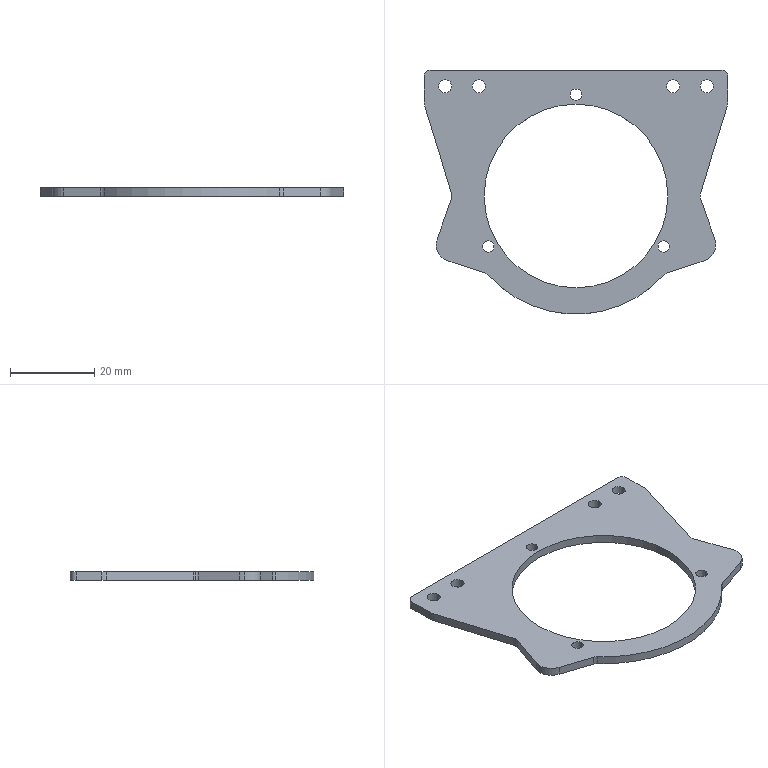Part | SolidWorks | features Fillet 3, Extrusion 1 | 1 solid | 40 faces | box 72 x 57.8 x 2 mm | volume 3745 mm3 | cylinder 29 | plane 11 | commonest cylinder face diameters 3.1 x8 2.7 x6 4 x5 8 x5 3 x2 43.5 x2
STEP:
#1=CARTESIAN_POINT('',(-33.109,-11.571,2.));
#2=VERTEX_POINT('',#1);
#3=CARTESIAN_POINT('',(-30.345,-15.376,2.));
#4=VERTEX_POINT('',#3);
#5=CARTESIAN_POINT('',(-29.109,-11.571,2.));
#6=DIRECTION('',(0.,0.,1.));
#7=DIRECTION('',(1.,0.,0.));
#8=AXIS2_PLACEMENT_3D('',#5,#6,#7);
#9=CIRCLE('',#8,4.);
#10=EDGE_CURVE('',#2,#4,#9,.T.);
#11=ORIENTED_EDGE('',*,*,#10,.F.);
#12=CARTESIAN_POINT('',(-33.109,-11.571,0.));
#13=VERTEX_POINT('',#12);
#14=CARTESIAN_POINT('',(-33.109,-11.571,2.));
#15=DIRECTION('',(0.,0.,-1.));
#16=VECTOR('',#15,1000.);
#17=LINE('',#14,#16);
#18=EDGE_CURVE('',#2,#13,#17,.T.);
#19=ORIENTED_EDGE('',*,*,#18,.T.);
#20=CARTESIAN_POINT('',(-30.345,-15.376,0.));
#21=VERTEX_POINT('',#20);
#22=CARTESIAN_POINT('',(-29.109,-11.571,0.));
#23=DIRECTION('',(0.,0.,-1.));
#24=DIRECTION('',(1.,0.,0.));
#25=AXIS2_PLACEMENT_3D('',#22,#23,#24);
#26=CIRCLE('',#25,4.);
#27=EDGE_CURVE('',#21,#13,#26,.T.);
#28=ORIENTED_EDGE('',*,*,#27,.F.);
#29=CARTESIAN_POINT('',(-30.345,-15.376,2.));
#30=DIRECTION('',(0.,0.,-1.));
#31=VECTOR('',#30,1000.);
#32=LINE('',#29,#31);
#33=EDGE_CURVE('',#4,#21,#32,.T.);
#34=ORIENTED_EDGE('',*,*,#33,.F.);
#35=EDGE_LOOP('',(#11,#19,#28,#34));
#36=FACE_OUTER_BOUND('',#35,.T.);
#37=CARTESIAN_POINT('',(-29.109,-11.571,2.));
#38=DIRECTION('',(0.,0.,-1.));
#39=DIRECTION('',(-1.,0.,0.));
#40=AXIS2_PLACEMENT_3D('',#37,#38,#39);
#41=CYLINDRICAL_SURFACE('',#40,4.);
#42=ADVANCED_FACE('',(#36),#41,.T.);
#43=CARTESIAN_POINT('',(-29.4,0.04046,0.));
#44=VERTEX_POINT('',#43);
#45=CARTESIAN_POINT('',(-29.488,0.6284,0.));
#46=VERTEX_POINT('',#45);
#47=CARTESIAN_POINT('',(-31.4,0.04046,0.));
#48=DIRECTION('',(0.,0.,1.));
#49=DIRECTION('',(1.,0.,0.));
#50=AXIS2_PLACEMENT_3D('',#47,#48,#49);
#51=CIRCLE('',#50,2.);
#52=EDGE_CURVE('',#44,#46,#51,.T.);
#53=ORIENTED_EDGE('',*,*,#52,.F.);
#54=CARTESIAN_POINT('',(-29.4,0.04046,2.));
#55=VERTEX_POINT('',#54);
#56=CARTESIAN_POINT('',(-29.4,0.04046,2.));
#57=DIRECTION('',(0.,0.,1.));
#58=VECTOR('',#57,1000.);
#59=LINE('',#56,#58);
#60=EDGE_CURVE('',#44,#55,#59,.T.);
#61=ORIENTED_EDGE('',*,*,#60,.T.);
#62=CARTESIAN_POINT('',(-29.488,0.6284,2.));
#63=VERTEX_POINT('',#62);
#64=CARTESIAN_POINT('',(-31.4,0.04046,2.));
#65=DIRECTION('',(0.,0.,-1.));
#66=DIRECTION('',(1.,0.,0.));
#67=AXIS2_PLACEMENT_3D('',#64,#65,#66);
#68=CIRCLE('',#67,2.);
#69=EDGE_CURVE('',#63,#55,#68,.T.);
#70=ORIENTED_EDGE('',*,*,#69,.F.);
#71=CARTESIAN_POINT('',(-29.488,0.6284,2.));
#72=DIRECTION('',(0.,0.,1.));
#73=VECTOR('',#72,1000.);
#74=LINE('',#71,#73);
#75=EDGE_CURVE('',#46,#63,#74,.T.);
#76=ORIENTED_EDGE('',*,*,#75,.F.);
#77=EDGE_LOOP('',(#53,#61,#70,#76));
#78=FACE_OUTER_BOUND('',#77,.T.);
#79=CARTESIAN_POINT('',(-31.4,0.04046,2.));
#80=DIRECTION('',(0.,0.,1.));
#81=DIRECTION('',(1.,0.,0.));
#82=AXIS2_PLACEMENT_3D('',#79,#80,#81);
#83=CYLINDRICAL_SURFACE('',#82,2.);
#84=ADVANCED_FACE('',(#78),#83,.F.);
#85=CARTESIAN_POINT('',(-22.135,-12.,2.));
#86=VERTEX_POINT('',#85);
#87=CARTESIAN_POINT('',(-19.435,-12.,2.));
#88=VERTEX_POINT('',#87);
#89=CARTESIAN_POINT('',(-20.785,-12.,2.));
#90=DIRECTION('',(0.,0.,1.));
#91=DIRECTION('',(1.,0.,0.));
#92=AXIS2_PLACEMENT_3D('',#89,#90,#91);
#93=CIRCLE('',#92,1.35);
#94=EDGE_CURVE('',#86,#88,#93,.T.);
#95=ORIENTED_EDGE('',*,*,#94,.T.);
#96=CARTESIAN_POINT('',(-19.435,-12.,0.));
#97=VERTEX_POINT('',#96);
#98=CARTESIAN_POINT('',(-19.435,-12.,2.));
#99=DIRECTION('',(0.,0.,-1.));
#100=VECTOR('',#99,1000.);
#101=LINE('',#98,#100);
#102=EDGE_CURVE('',#88,#97,#101,.T.);
#103=ORIENTED_EDGE('',*,*,#102,.T.);
#104=CARTESIAN_POINT('',(-22.135,-12.,0.));
#105=VERTEX_POINT('',#104);
#106=CARTESIAN_POINT('',(-20.785,-12.,0.));
#107=DIRECTION('',(0.,0.,1.));
#108=DIRECTION('',(1.,0.,0.));
#109=AXIS2_PLACEMENT_3D('',#106,#107,#108);
#110=CIRCLE('',#109,1.35);
#111=EDGE_CURVE('',#105,#97,#110,.T.);
#112=ORIENTED_EDGE('',*,*,#111,.F.);
#113=CARTESIAN_POINT('',(-22.135,-12.,2.));
#114=DIRECTION('',(0.,0.,-1.));
#115=VECTOR('',#114,1000.);
#116=LINE('',#113,#115);
#117=EDGE_CURVE('',#86,#105,#116,.T.);
#118=ORIENTED_EDGE('',*,*,#117,.F.);
#119=EDGE_LOOP('',(#95,#103,#112,#118));
#120=FACE_OUTER_BOUND('',#119,.T.);
#121=CARTESIAN_POINT('',(-20.785,-12.,2.));
#122=DIRECTION('',(0.,0.,-1.));
#123=DIRECTION('',(-1.,0.,0.));
#124=AXIS2_PLACEMENT_3D('',#121,#122,#123);
#125=CYLINDRICAL_SURFACE('',#124,1.35);
#126=ADVANCED_FACE('',(#120),#125,.F.);
#127=CARTESIAN_POINT('',(19.435,-12.,2.));
#128=VERTEX_POINT('',#127);
#129=CARTESIAN_POINT('',(22.135,-12.,2.));
#130=VERTEX_POINT('',#129);
#131=CARTESIAN_POINT('',(20.785,-12.,2.));
#132=DIRECTION('',(0.,0.,1.));
#133=DIRECTION('',(1.,0.,0.));
#134=AXIS2_PLACEMENT_3D('',#131,#132,#133);
#135=CIRCLE('',#134,1.35);
#136=EDGE_CURVE('',#128,#130,#135,.T.);
#137=ORIENTED_EDGE('',*,*,#136,.T.);
#138=CARTESIAN_POINT('',(22.135,-12.,0.));
#139=VERTEX_POINT('',#138);
#140=CARTESIAN_POINT('',(22.135,-12.,2.));
#141=DIRECTION('',(0.,0.,-1.));
#142=VECTOR('',#141,1000.);
#143=LINE('',#140,#142);
#144=EDGE_CURVE('',#130,#139,#143,.T.);
#145=ORIENTED_EDGE('',*,*,#144,.T.);
#146=CARTESIAN_POINT('',(19.435,-12.,0.));
#147=VERTEX_POINT('',#146);
#148=CARTESIAN_POINT('',(20.785,-12.,0.));
#149=DIRECTION('',(0.,0.,1.));
#150=DIRECTION('',(1.,0.,0.));
#151=AXIS2_PLACEMENT_3D('',#148,#149,#150);
#152=CIRCLE('',#151,1.35);
#153=EDGE_CURVE('',#147,#139,#152,.T.);
#154=ORIENTED_EDGE('',*,*,#153,.F.);
#155=CARTESIAN_POINT('',(19.435,-12.,2.));
#156=DIRECTION('',(0.,0.,-1.));
#157=VECTOR('',#156,1000.);
#158=LINE('',#155,#157);
#159=EDGE_CURVE('',#128,#147,#158,.T.);
#160=ORIENTED_EDGE('',*,*,#159,.F.);
#161=EDGE_LOOP('',(#137,#145,#154,#160));
#162=FACE_OUTER_BOUND('',#161,.T.);
#163=CARTESIAN_POINT('',(20.785,-12.,2.));
#164=DIRECTION('',(0.,0.,-1.));
#165=DIRECTION('',(-1.,0.,0.));
#166=AXIS2_PLACEMENT_3D('',#163,#164,#165);
#167=CYLINDRICAL_SURFACE('',#166,1.35);
#168=ADVANCED_FACE('',(#162),#167,.F.);
#169=CARTESIAN_POINT('',(29.45,26.,2.));
#170=VERTEX_POINT('',#169);
#171=CARTESIAN_POINT('',(32.55,26.,2.));
#172=VERTEX_POINT('',#171);
#173=CARTESIAN_POINT('',(31.,26.,2.));
#174=DIRECTION('',(0.,0.,1.));
#175=DIRECTION('',(-1.,0.,0.));
#176=AXIS2_PLACEMENT_3D('',#173,#174,#175);
#177=CIRCLE('',#176,1.55);
#178=EDGE_CURVE('',#170,#172,#177,.T.);
#179=ORIENTED_EDGE('',*,*,#178,.T.);
#180=CARTESIAN_POINT('',(32.55,26.,0.));
#181=VERTEX_POINT('',#180);
#182=CARTESIAN_POINT('',(32.55,26.,2.));
#183=DIRECTION('',(0.,0.,-1.));
#184=VECTOR('',#183,1000.);
#185=LINE('',#182,#184);
#186=EDGE_CURVE('',#172,#181,#185,.T.);
#187=ORIENTED_EDGE('',*,*,#186,.T.);
#188=CARTESIAN_POINT('',(29.45,26.,0.));
#189=VERTEX_POINT('',#188);
#190=CARTESIAN_POINT('',(31.,26.,0.));
#191=DIRECTION('',(0.,0.,1.));
#192=DIRECTION('',(-1.,0.,0.));
#193=AXIS2_PLACEMENT_3D('',#190,#191,#192);
#194=CIRCLE('',#193,1.55);
#195=EDGE_CURVE('',#189,#181,#194,.T.);
#196=ORIENTED_EDGE('',*,*,#195,.F.);
#197=CARTESIAN_POINT('',(29.45,26.,2.));
#198=DIRECTION('',(0.,0.,-1.));
#199=VECTOR('',#198,1000.);
#200=LINE('',#197,#199);
#201=EDGE_CURVE('',#170,#189,#200,.T.);
#202=ORIENTED_EDGE('',*,*,#201,.F.);
#203=EDGE_LOOP('',(#179,#187,#196,#202));
#204=FACE_OUTER_BOUND('',#203,.T.);
#205=CARTESIAN_POINT('',(31.,26.,2.));
#206=DIRECTION('',(0.,0.,-1.));
#207=DIRECTION('',(-1.,0.,0.));
#208=AXIS2_PLACEMENT_3D('',#205,#206,#207);
#209=CYLINDRICAL_SURFACE('',#208,1.55);
#210=ADVANCED_FACE('',(#204),#209,.F.);
#211=CARTESIAN_POINT('',(21.45,26.,2.));
#212=VERTEX_POINT('',#211);
#213=CARTESIAN_POINT('',(24.55,26.,2.));
#214=VERTEX_POINT('',#213);
#215=CARTESIAN_POINT('',(23.,26.,2.));
#216=DIRECTION('',(0.,0.,1.));
#217=DIRECTION('',(-1.,0.,0.));
#218=AXIS2_PLACEMENT_3D('',#215,#216,#217);
#219=CIRCLE('',#218,1.55);
#220=EDGE_CURVE('',#212,#214,#219,.T.);
#221=ORIENTED_EDGE('',*,*,#220,.T.);
#222=CARTESIAN_POINT('',(24.55,26.,0.));
#223=VERTEX_POINT('',#222);
#224=CARTESIAN_POINT('',(24.55,26.,2.));
#225=DIRECTION('',(0.,0.,-1.));
#226=VECTOR('',#225,1000.);
#227=LINE('',#224,#226);
#228=EDGE_CURVE('',#214,#223,#227,.T.);
#229=ORIENTED_EDGE('',*,*,#228,.T.);
#230=CARTESIAN_POINT('',(21.45,26.,0.));
#231=VERTEX_POINT('',#230);
#232=CARTESIAN_POINT('',(23.,26.,0.));
#233=DIRECTION('',(0.,0.,1.));
#234=DIRECTION('',(-1.,0.,0.));
#235=AXIS2_PLACEMENT_3D('',#232,#233,#234);
#236=CIRCLE('',#235,1.55);
#237=EDGE_CURVE('',#231,#223,#236,.T.);
#238=ORIENTED_EDGE('',*,*,#237,.F.);
#239=CARTESIAN_POINT('',(21.45,26.,2.));
#240=DIRECTION('',(0.,0.,-1.));
#241=VECTOR('',#240,1000.);
#242=LINE('',#239,#241);
#243=EDGE_CURVE('',#212,#231,#242,.T.);
#244=ORIENTED_EDGE('',*,*,#243,.F.);
#245=EDGE_LOOP('',(#221,#229,#238,#244));
#246=FACE_OUTER_BOUND('',#245,.T.);
#247=CARTESIAN_POINT('',(23.,26.,2.));
#248=DIRECTION('',(0.,0.,-1.));
#249=DIRECTION('',(-1.,0.,0.));
#250=AXIS2_PLACEMENT_3D('',#247,#248,#249);
#251=CYLINDRICAL_SURFACE('',#250,1.55);
#252=ADVANCED_FACE('',(#246),#251,.F.);
#253=CARTESIAN_POINT('',(-32.55,26.,2.));
#254=VERTEX_POINT('',#253);
#255=CARTESIAN_POINT('',(-29.45,26.,2.));
#256=VERTEX_POINT('',#255);
#257=CARTESIAN_POINT('',(-31.,26.,2.));
#258=DIRECTION('',(0.,0.,1.));
#259=DIRECTION('',(1.,0.,0.));
#260=AXIS2_PLACEMENT_3D('',#257,#258,#259);
#261=CIRCLE('',#260,1.55);
#262=EDGE_CURVE('',#254,#256,#261,.T.);
#263=ORIENTED_EDGE('',*,*,#262,.T.);
#264=CARTESIAN_POINT('',(-29.45,26.,0.));
#265=VERTEX_POINT('',#264);
#266=CARTESIAN_POINT('',(-29.45,26.,2.));
#267=DIRECTION('',(0.,0.,-1.));
#268=VECTOR('',#267,1000.);
#269=LINE('',#266,#268);
#270=EDGE_CURVE('',#256,#265,#269,.T.);
#271=ORIENTED_EDGE('',*,*,#270,.T.);
#272=CARTESIAN_POINT('',(-32.55,26.,0.));
#273=VERTEX_POINT('',#272);
#274=CARTESIAN_POINT('',(-31.,26.,0.));
#275=DIRECTION('',(0.,0.,1.));
#276=DIRECTION('',(1.,0.,0.));
#277=AXIS2_PLACEMENT_3D('',#274,#275,#276);
#278=CIRCLE('',#277,1.55);
#279=EDGE_CURVE('',#273,#265,#278,.T.);
#280=ORIENTED_EDGE('',*,*,#279,.F.);
#281=CARTESIAN_POINT('',(-32.55,26.,2.));
#282=DIRECTION('',(0.,0.,-1.));
#283=VECTOR('',#282,1000.);
#284=LINE('',#281,#283);
#285=EDGE_CURVE('',#254,#273,#284,.T.);
#286=ORIENTED_EDGE('',*,*,#285,.F.);
#287=EDGE_LOOP('',(#263,#271,#280,#286));
#288=FACE_OUTER_BOUND('',#287,.T.);
#289=CARTESIAN_POINT('',(-31.,26.,2.));
#290=DIRECTION('',(0.,0.,-1.));
#291=DIRECTION('',(-1.,0.,0.));
#292=AXIS2_PLACEMENT_3D('',#289,#290,#291);
#293=CYLINDRICAL_SURFACE('',#292,1.55);
#294=ADVANCED_FACE('',(#288),#293,.F.);
#295=CARTESIAN_POINT('',(-24.55,26.,2.));
#296=VERTEX_POINT('',#295);
#297=CARTESIAN_POINT('',(-21.45,26.,2.));
#298=VERTEX_POINT('',#297);
#299=CARTESIAN_POINT('',(-23.,26.,2.));
#300=DIRECTION('',(0.,0.,1.));
#301=DIRECTION('',(1.,0.,0.));
#302=AXIS2_PLACEMENT_3D('',#299,#300,#301);
#303=CIRCLE('',#302,1.55);
#304=EDGE_CURVE('',#296,#298,#303,.T.);
#305=ORIENTED_EDGE('',*,*,#304,.T.);
#306=CARTESIAN_POINT('',(-21.45,26.,0.));
#307=VERTEX_POINT('',#306);
#308=CARTESIAN_POINT('',(-21.45,26.,2.));
#309=DIRECTION('',(0.,0.,-1.));
#310=VECTOR('',#309,1000.);
#311=LINE('',#308,#310);
#312=EDGE_CURVE('',#298,#307,#311,.T.);
#313=ORIENTED_EDGE('',*,*,#312,.T.);
#314=CARTESIAN_POINT('',(-24.55,26.,0.));
#315=VERTEX_POINT('',#314);
#316=CARTESIAN_POINT('',(-23.,26.,0.));
#317=DIRECTION('',(0.,0.,1.));
#318=DIRECTION('',(1.,0.,0.));
#319=AXIS2_PLACEMENT_3D('',#316,#317,#318);
#320=CIRCLE('',#319,1.55);
#321=EDGE_CURVE('',#315,#307,#320,.T.);
#322=ORIENTED_EDGE('',*,*,#321,.F.);
#323=CARTESIAN_POINT('',(-24.55,26.,2.));
#324=DIRECTION('',(0.,0.,-1.));
#325=VECTOR('',#324,1000.);
#326=LINE('',#323,#325);
#327=EDGE_CURVE('',#296,#315,#326,.T.);
#328=ORIENTED_EDGE('',*,*,#327,.F.);
#329=EDGE_LOOP('',(#305,#313,#322,#328));
#330=FACE_OUTER_BOUND('',#329,.T.);
#331=CARTESIAN_POINT('',(-23.,26.,2.));
#332=DIRECTION('',(0.,0.,-1.));
#333=DIRECTION('',(-1.,0.,0.));
#334=AXIS2_PLACEMENT_3D('',#331,#332,#333);
#335=CYLINDRICAL_SURFACE('',#334,1.55);
#336=ADVANCED_FACE('',(#330),#335,.F.);
#337=CARTESIAN_POINT('',(-21.75,0.,2.));
#338=VERTEX_POINT('',#337);
#339=CARTESIAN_POINT('',(21.75,0.,2.));
#340=VERTEX_POINT('',#339);
#341=CARTESIAN_POINT('',(0.,0.,2.));
#342=DIRECTION('',(0.,0.,1.));
#343=DIRECTION('',(1.,0.,0.));
#344=AXIS2_PLACEMENT_3D('',#341,#342,#343);
#345=CIRCLE('',#344,21.75);
#346=EDGE_CURVE('',#338,#340,#345,.T.);
#347=ORIENTED_EDGE('',*,*,#346,.T.);
#348=CARTESIAN_POINT('',(21.75,0.,0.));
#349=VERTEX_POINT('',#348);
#350=CARTESIAN_POINT('',(21.75,0.,2.));
#351=DIRECTION('',(0.,0.,-1.));
#352=VECTOR('',#351,1000.);
#353=LINE('',#350,#352);
#354=EDGE_CURVE('',#340,#349,#353,.T.);
#355=ORIENTED_EDGE('',*,*,#354,.T.);
#356=CARTESIAN_POINT('',(-21.75,0.,0.));
#357=VERTEX_POINT('',#356);
#358=CARTESIAN_POINT('',(0.,0.,0.));
#359=DIRECTION('',(0.,0.,1.));
#360=DIRECTION('',(1.,0.,0.));
#361=AXIS2_PLACEMENT_3D('',#358,#359,#360);
#362=CIRCLE('',#361,21.75);
#363=EDGE_CURVE('',#357,#349,#362,.T.);
#364=ORIENTED_EDGE('',*,*,#363,.F.);
#365=CARTESIAN_POINT('',(-21.75,0.,2.));
#366=DIRECTION('',(0.,0.,-1.));
#367=VECTOR('',#366,1000.);
#368=LINE('',#365,#367);
#369=EDGE_CURVE('',#338,#357,#368,.T.);
#370=ORIENTED_EDGE('',*,*,#369,.F.);
#371=EDGE_LOOP('',(#347,#355,#364,#370));
#372=FACE_OUTER_BOUND('',#371,.T.);
#373=CARTESIAN_POINT('',(0.,0.,2.));
#374=DIRECTION('',(0.,0.,-1.));
#375=DIRECTION('',(-1.,0.,0.));
#376=AXIS2_PLACEMENT_3D('',#373,#374,#375);
#377=CYLINDRICAL_SURFACE('',#376,21.75);
#378=ADVANCED_FACE('',(#372),#377,.F.);
#379=CARTESIAN_POINT('',(-1.35,24.,2.));
#380=VERTEX_POINT('',#379);
#381=CARTESIAN_POINT('',(1.35,24.,2.));
#382=VERTEX_POINT('',#381);
#383=CARTESIAN_POINT('',(0.,24.,2.));
#384=DIRECTION('',(0.,0.,1.));
#385=DIRECTION('',(1.,0.,0.));
#386=AXIS2_PLACEMENT_3D('',#383,#384,#385);
#387=CIRCLE('',#386,1.35);
#388=EDGE_CURVE('',#380,#382,#387,.T.);
#389=ORIENTED_EDGE('',*,*,#388,.T.);
#390=CARTESIAN_POINT('',(1.35,24.,0.));
#391=VERTEX_POINT('',#390);
#392=CARTESIAN_POINT('',(1.35,24.,2.));
#393=DIRECTION('',(0.,0.,-1.));
#394=VECTOR('',#393,1000.);
#395=LINE('',#392,#394);
#396=EDGE_CURVE('',#382,#391,#395,.T.);
#397=ORIENTED_EDGE('',*,*,#396,.T.);
#398=CARTESIAN_POINT('',(-1.35,24.,0.));
#399=VERTEX_POINT('',#398);
#400=CARTESIAN_POINT('',(0.,24.,0.));
#401=DIRECTION('',(0.,0.,1.));
#402=DIRECTION('',(1.,0.,0.));
#403=AXIS2_PLACEMENT_3D('',#400,#401,#402);
#404=CIRCLE('',#403,1.35);
#405=EDGE_CURVE('',#399,#391,#404,.T.);
#406=ORIENTED_EDGE('',*,*,#405,.F.);
#407=CARTESIAN_POINT('',(-1.35,24.,2.));
#408=DIRECTION('',(0.,0.,-1.));
#409=VECTOR('',#408,1000.);
#410=LINE('',#407,#409);
#411=EDGE_CURVE('',#380,#399,#410,.T.);
#412=ORIENTED_EDGE('',*,*,#411,.F.);
#413=EDGE_LOOP('',(#389,#397,#406,#412));
#414=FACE_OUTER_BOUND('',#413,.T.);
#415=CARTESIAN_POINT('',(0.,24.,2.));
#416=DIRECTION('',(0.,0.,-1.));
#417=DIRECTION('',(-1.,0.,0.));
#418=AXIS2_PLACEMENT_3D('',#415,#416,#417);
#419=CYLINDRICAL_SURFACE('',#418,1.35);
#420=ADVANCED_FACE('',(#414),#419,.F.);
#421=ORIENTED_EDGE('',*,*,#136,.F.);
#422=CARTESIAN_POINT('',(20.785,-12.,2.));
#423=DIRECTION('',(0.,0.,1.));
#424=DIRECTION('',(1.,0.,0.));
#425=AXIS2_PLACEMENT_3D('',#422,#423,#424);
#426=CIRCLE('',#425,1.35);
#427=EDGE_CURVE('',#130,#128,#426,.T.);
#428=ORIENTED_EDGE('',*,*,#427,.F.);
#429=EDGE_LOOP('',(#421,#428));
#430=FACE_BOUND('',#429,.T.);
#431=ORIENTED_EDGE('',*,*,#220,.F.);
#432=CARTESIAN_POINT('',(23.,26.,2.));
#433=DIRECTION('',(0.,0.,1.));
#434=DIRECTION('',(-1.,0.,0.));
#435=AXIS2_PLACEMENT_3D('',#432,#433,#434);
#436=CIRCLE('',#435,1.55);
#437=EDGE_CURVE('',#214,#212,#436,.T.);
#438=ORIENTED_EDGE('',*,*,#437,.F.);
#439=EDGE_LOOP('',(#431,#438));
#440=FACE_BOUND('',#439,.T.);
#441=ORIENTED_EDGE('',*,*,#304,.F.);
#442=CARTESIAN_POINT('',(-23.,26.,2.));
#443=DIRECTION('',(0.,0.,1.));
#444=DIRECTION('',(1.,0.,0.));
#445=AXIS2_PLACEMENT_3D('',#442,#443,#444);
#446=CIRCLE('',#445,1.55);
#447=EDGE_CURVE('',#298,#296,#446,.T.);
#448=ORIENTED_EDGE('',*,*,#447,.F.);
#449=EDGE_LOOP('',(#441,#448));
#450=FACE_BOUND('',#449,.T.);
#451=ORIENTED_EDGE('',*,*,#388,.F.);
#452=CARTESIAN_POINT('',(0.,24.,2.));
#453=DIRECTION('',(0.,0.,1.));
#454=DIRECTION('',(1.,0.,0.));
#455=AXIS2_PLACEMENT_3D('',#452,#453,#454);
#456=CIRCLE('',#455,1.35);
#457=EDGE_CURVE('',#382,#380,#456,.T.);
#458=ORIENTED_EDGE('',*,*,#457,.F.);
#459=EDGE_LOOP('',(#451,#458));
#460=FACE_BOUND('',#459,.T.);
#461=CARTESIAN_POINT('',(36.,22.401,2.));
#462=VERTEX_POINT('',#461);
#463=CARTESIAN_POINT('',(36.,28.3,2.));
#464=VERTEX_POINT('',#463);
#465=CARTESIAN_POINT('',(36.,29.8,2.));
#466=DIRECTION('',(0.,1.,0.));
#467=VECTOR('',#466,1000.);
#468=LINE('',#465,#467);
#469=EDGE_CURVE('',#462,#464,#468,.T.);
#470=ORIENTED_EDGE('',*,*,#469,.T.);
#471=CARTESIAN_POINT('',(34.5,29.8,2.));
#472=VERTEX_POINT('',#471);
#473=CARTESIAN_POINT('',(34.5,28.3,2.));
#474=DIRECTION('',(0.,0.,1.));
#475=DIRECTION('',(1.,0.,0.));
#476=AXIS2_PLACEMENT_3D('',#473,#474,#475);
#477=CIRCLE('',#476,1.5);
#478=EDGE_CURVE('',#464,#472,#477,.T.);
#479=ORIENTED_EDGE('',*,*,#478,.T.);
#480=CARTESIAN_POINT('',(-34.5,29.8,2.));
#481=VERTEX_POINT('',#480);
#482=CARTESIAN_POINT('',(36.,29.8,2.));
#483=DIRECTION('',(-1.,0.,0.));
#484=VECTOR('',#483,1000.);
#485=LINE('',#482,#484);
#486=EDGE_CURVE('',#472,#481,#485,.T.);
#487=ORIENTED_EDGE('',*,*,#486,.T.);
#488=CARTESIAN_POINT('',(-36.,28.3,2.));
#489=VERTEX_POINT('',#488);
#490=CARTESIAN_POINT('',(-34.5,28.3,2.));
#491=DIRECTION('',(0.,0.,1.));
#492=DIRECTION('',(1.,0.,0.));
#493=AXIS2_PLACEMENT_3D('',#490,#491,#492);
#494=CIRCLE('',#493,1.5);
#495=EDGE_CURVE('',#481,#489,#494,.T.);
#496=ORIENTED_EDGE('',*,*,#495,.T.);
#497=CARTESIAN_POINT('',(-36.,22.401,2.));
#498=VERTEX_POINT('',#497);
#499=CARTESIAN_POINT('',(-36.,29.8,2.));
#500=DIRECTION('',(0.,-1.,0.));
#501=VECTOR('',#500,1000.);
#502=LINE('',#499,#501);
#503=EDGE_CURVE('',#489,#498,#502,.T.);
#504=ORIENTED_EDGE('',*,*,#503,.T.);
#505=CARTESIAN_POINT('',(-35.823,21.225,2.));
#506=VERTEX_POINT('',#505);
#507=CARTESIAN_POINT('',(-32.,22.401,2.));
#508=DIRECTION('',(0.,0.,1.));
#509=DIRECTION('',(1.,0.,0.));
#510=AXIS2_PLACEMENT_3D('',#507,#508,#509);
#511=CIRCLE('',#510,4.);
#512=EDGE_CURVE('',#498,#506,#511,.T.);
#513=ORIENTED_EDGE('',*,*,#512,.T.);
#514=CARTESIAN_POINT('',(-36.,21.8,2.));
#515=DIRECTION('',(0.294,-0.9558,0.));
#516=VECTOR('',#515,1000.);
#517=LINE('',#514,#516);
#518=EDGE_CURVE('',#506,#63,#517,.T.);
#519=ORIENTED_EDGE('',*,*,#518,.T.);
#520=ORIENTED_EDGE('',*,*,#69,.T.);
#521=CARTESIAN_POINT('',(-29.512,-0.6206,2.));
#522=VERTEX_POINT('',#521);
#523=CARTESIAN_POINT('',(-31.4,0.04046,2.));
#524=DIRECTION('',(0.,0.,-1.));
#525=DIRECTION('',(1.,0.,0.));
#526=AXIS2_PLACEMENT_3D('',#523,#524,#525);
#527=CIRCLE('',#526,2.);
#528=EDGE_CURVE('',#55,#522,#527,.T.);
#529=ORIENTED_EDGE('',*,*,#528,.T.);
#530=CARTESIAN_POINT('',(-32.884,-10.249,2.));
#531=VERTEX_POINT('',#530);
#532=CARTESIAN_POINT('',(-29.295,0.,2.));
#533=DIRECTION('',(-0.3305,-0.9438,0.));
#534=VECTOR('',#533,1000.);
#535=LINE('',#532,#534);
#536=EDGE_CURVE('',#522,#531,#535,.T.);
#537=ORIENTED_EDGE('',*,*,#536,.T.);
#538=CARTESIAN_POINT('',(-29.109,-11.571,2.));
#539=DIRECTION('',(0.,0.,1.));
#540=DIRECTION('',(1.,0.,0.));
#541=AXIS2_PLACEMENT_3D('',#538,#539,#540);
#542=CIRCLE('',#541,4.);
#543=EDGE_CURVE('',#531,#2,#542,.T.);
#544=ORIENTED_EDGE('',*,*,#543,.T.);
#545=ORIENTED_EDGE('',*,*,#10,.T.);
#546=CARTESIAN_POINT('',(-21.651,-18.2,2.));
#547=VERTEX_POINT('',#546);
#548=CARTESIAN_POINT('',(-34.236,-14.111,2.));
#549=DIRECTION('',(0.9511,-0.309,0.));
#550=VECTOR('',#549,1000.);
#551=LINE('',#548,#550);
#552=EDGE_CURVE('',#4,#547,#551,.T.);
#553=ORIENTED_EDGE('',*,*,#552,.T.);
#554=CARTESIAN_POINT('',(-20.784,-18.762,2.));
#555=VERTEX_POINT('',#554);
#556=CARTESIAN_POINT('',(-22.269,-20.103,2.));
#557=DIRECTION('',(0.,0.,-1.));
#558=DIRECTION('',(1.,0.,0.));
#559=AXIS2_PLACEMENT_3D('',#556,#557,#558);
#560=CIRCLE('',#559,2.);
#561=EDGE_CURVE('',#547,#555,#560,.T.);
#562=ORIENTED_EDGE('',*,*,#561,.T.);
#563=CARTESIAN_POINT('',(20.784,-18.762,2.));
#564=VERTEX_POINT('',#563);
#565=CARTESIAN_POINT('',(0.,0.,2.));
#566=DIRECTION('',(0.,0.,1.));
#567=DIRECTION('',(1.,0.,0.));
#568=AXIS2_PLACEMENT_3D('',#565,#566,#567);
#569=CIRCLE('',#568,28.);
#570=EDGE_CURVE('',#555,#564,#569,.T.);
#571=ORIENTED_EDGE('',*,*,#570,.T.);
#572=CARTESIAN_POINT('',(21.651,-18.2,2.));
#573=VERTEX_POINT('',#572);
#574=CARTESIAN_POINT('',(22.269,-20.103,2.));
#575=DIRECTION('',(0.,0.,-1.));
#576=DIRECTION('',(1.,0.,0.));
#577=AXIS2_PLACEMENT_3D('',#574,#575,#576);
#578=CIRCLE('',#577,2.);
#579=EDGE_CURVE('',#564,#573,#578,.T.);
#580=ORIENTED_EDGE('',*,*,#579,.T.);
#581=CARTESIAN_POINT('',(30.345,-15.376,2.));
#582=VERTEX_POINT('',#581);
#583=CARTESIAN_POINT('',(34.236,-14.111,2.));
#584=DIRECTION('',(0.9511,0.309,0.));
#585=VECTOR('',#584,1000.);
#586=LINE('',#583,#585);
#587=EDGE_CURVE('',#573,#582,#586,.T.);
#588=ORIENTED_EDGE('',*,*,#587,.T.);
#589=CARTESIAN_POINT('',(32.884,-10.249,2.));
#590=VERTEX_POINT('',#589);
#591=CARTESIAN_POINT('',(29.109,-11.571,2.));
#592=DIRECTION('',(0.,0.,1.));
#593=DIRECTION('',(1.,0.,0.));
#594=AXIS2_PLACEMENT_3D('',#591,#592,#593);
#595=CIRCLE('',#594,4.);
#596=EDGE_CURVE('',#582,#590,#595,.T.);
#597=ORIENTED_EDGE('',*,*,#596,.T.);
#598=CARTESIAN_POINT('',(29.512,-0.6206,2.));
#599=VERTEX_POINT('',#598);
#600=CARTESIAN_POINT('',(29.295,0.,2.));
#601=DIRECTION('',(-0.3305,0.9438,0.));
#602=VECTOR('',#601,1000.);
#603=LINE('',#600,#602);
#604=EDGE_CURVE('',#590,#599,#603,.T.);
#605=ORIENTED_EDGE('',*,*,#604,.T.);
#606=CARTESIAN_POINT('',(29.488,0.6284,2.));
#607=VERTEX_POINT('',#606);
#608=CARTESIAN_POINT('',(31.4,0.04046,2.));
#609=DIRECTION('',(0.,0.,-1.));
#610=DIRECTION('',(1.,0.,0.));
#611=AXIS2_PLACEMENT_3D('',#608,#609,#610);
#612=CIRCLE('',#611,2.);
#613=EDGE_CURVE('',#599,#607,#612,.T.);
#614=ORIENTED_EDGE('',*,*,#613,.T.);
#615=CARTESIAN_POINT('',(35.823,21.225,2.));
#616=VERTEX_POINT('',#615);
#617=CARTESIAN_POINT('',(36.,21.8,2.));
#618=DIRECTION('',(0.294,0.9558,0.));
#619=VECTOR('',#618,1000.);
#620=LINE('',#617,#619);
#621=EDGE_CURVE('',#607,#616,#620,.T.);
#622=ORIENTED_EDGE('',*,*,#621,.T.);
#623=CARTESIAN_POINT('',(32.,22.401,2.));
#624=DIRECTION('',(0.,0.,1.));
#625=DIRECTION('',(1.,0.,0.));
#626=AXIS2_PLACEMENT_3D('',#623,#624,#625);
#627=CIRCLE('',#626,4.);
#628=EDGE_CURVE('',#616,#462,#627,.T.);
#629=ORIENTED_EDGE('',*,*,#628,.T.);
#630=EDGE_LOOP('',(#470,#479,#487,#496,#504,#513,#519,#520,#529,#537,#544,#545,#553,#562,#571,#580,#588,#597,#605,#614,#622,#629));
#631=FACE_OUTER_BOUND('',#630,.T.);
#632=ORIENTED_EDGE('',*,*,#346,.F.);
#633=CARTESIAN_POINT('',(0.,0.,2.));
#634=DIRECTION('',(0.,0.,1.));
#635=DIRECTION('',(1.,0.,0.));
#636=AXIS2_PLACEMENT_3D('',#633,#634,#635);
#637=CIRCLE('',#636,21.75);
#638=EDGE_CURVE('',#340,#338,#637,.T.);
#639=ORIENTED_EDGE('',*,*,#638,.F.);
#640=EDGE_LOOP('',(#632,#639));
#641=FACE_BOUND('',#640,.T.);
#642=ORIENTED_EDGE('',*,*,#262,.F.);
#643=CARTESIAN_POINT('',(-31.,26.,2.));
#644=DIRECTION('',(0.,0.,1.));
#645=DIRECTION('',(1.,0.,0.));
#646=AXIS2_PLACEMENT_3D('',#643,#644,#645);
#647=CIRCLE('',#646,1.55);
#648=EDGE_CURVE('',#256,#254,#647,.T.);
#649=ORIENTED_EDGE('',*,*,#648,.F.);
#650=EDGE_LOOP('',(#642,#649));
#651=FACE_BOUND('',#650,.T.);
#652=ORIENTED_EDGE('',*,*,#178,.F.);
#653=CARTESIAN_POINT('',(31.,26.,2.));
#654=DIRECTION('',(0.,0.,1.));
#655=DIRECTION('',(-1.,0.,0.));
#656=AXIS2_PLACEMENT_3D('',#653,#654,#655);
#657=CIRCLE('',#656,1.55);
#658=EDGE_CURVE('',#172,#170,#657,.T.);
#659=ORIENTED_EDGE('',*,*,#658,.F.);
#660=EDGE_LOOP('',(#652,#659));
#661=FACE_BOUND('',#660,.T.);
#662=ORIENTED_EDGE('',*,*,#94,.F.);
#663=CARTESIAN_POINT('',(-20.785,-12.,2.));
#664=DIRECTION('',(0.,0.,1.));
#665=DIRECTION('',(1.,0.,0.));
#666=AXIS2_PLACEMENT_3D('',#663,#664,#665);
#667=CIRCLE('',#666,1.35);
#668=EDGE_CURVE('',#88,#86,#667,.T.);
#669=ORIENTED_EDGE('',*,*,#668,.F.);
#670=EDGE_LOOP('',(#662,#669));
#671=FACE_BOUND('',#670,.T.);
#672=CARTESIAN_POINT('',(0.,0.,2.));
#673=DIRECTION('',(0.,0.,1.));
#674=DIRECTION('',(1.,0.,0.));
#675=AXIS2_PLACEMENT_3D('',#672,#673,#674);
#676=PLANE('',#675);
#677=ADVANCED_FACE('',(#430,#440,#450,#460,#631,#641,#651,#661,#671),#676,.T.);
#678=CARTESIAN_POINT('',(34.5,29.8,0.));
#679=VERTEX_POINT('',#678);
#680=CARTESIAN_POINT('',(-34.5,29.8,0.));
#681=VERTEX_POINT('',#680);
#682=CARTESIAN_POINT('',(36.,29.8,0.));
#683=DIRECTION('',(-1.,0.,0.));
#684=VECTOR('',#683,1000.);
#685=LINE('',#682,#684);
#686=EDGE_CURVE('',#679,#681,#685,.T.);
#687=ORIENTED_EDGE('',*,*,#686,.F.);
#688=CARTESIAN_POINT('',(36.,28.3,0.));
#689=VERTEX_POINT('',#688);
#690=CARTESIAN_POINT('',(34.5,28.3,0.));
#691=DIRECTION('',(0.,0.,-1.));
#692=DIRECTION('',(1.,0.,0.));
#693=AXIS2_PLACEMENT_3D('',#690,#691,#692);
#694=CIRCLE('',#693,1.5);
#695=EDGE_CURVE('',#679,#689,#694,.T.);
#696=ORIENTED_EDGE('',*,*,#695,.T.);
#697=CARTESIAN_POINT('',(36.,22.401,0.));
#698=VERTEX_POINT('',#697);
#699=CARTESIAN_POINT('',(36.,29.8,0.));
#700=DIRECTION('',(0.,1.,0.));
#701=VECTOR('',#700,1000.);
#702=LINE('',#699,#701);
#703=EDGE_CURVE('',#698,#689,#702,.T.);
#704=ORIENTED_EDGE('',*,*,#703,.F.);
#705=CARTESIAN_POINT('',(35.823,21.225,0.));
#706=VERTEX_POINT('',#705);
#707=CARTESIAN_POINT('',(32.,22.401,0.));
#708=DIRECTION('',(0.,0.,-1.));
#709=DIRECTION('',(1.,0.,0.));
#710=AXIS2_PLACEMENT_3D('',#707,#708,#709);
#711=CIRCLE('',#710,4.);
#712=EDGE_CURVE('',#698,#706,#711,.T.);
#713=ORIENTED_EDGE('',*,*,#712,.T.);
#714=CARTESIAN_POINT('',(29.488,0.6284,0.));
#715=VERTEX_POINT('',#714);
#716=CARTESIAN_POINT('',(36.,21.8,0.));
#717=DIRECTION('',(0.294,0.9558,0.));
#718=VECTOR('',#717,1000.);
#719=LINE('',#716,#718);
#720=EDGE_CURVE('',#715,#706,#719,.T.);
#721=ORIENTED_EDGE('',*,*,#720,.F.);
#722=CARTESIAN_POINT('',(29.512,-0.6206,0.));
#723=VERTEX_POINT('',#722);
#724=CARTESIAN_POINT('',(31.4,0.04046,0.));
#725=DIRECTION('',(0.,0.,1.));
#726=DIRECTION('',(1.,0.,0.));
#727=AXIS2_PLACEMENT_3D('',#724,#725,#726);
#728=CIRCLE('',#727,2.);
#729=EDGE_CURVE('',#715,#723,#728,.T.);
#730=ORIENTED_EDGE('',*,*,#729,.T.);
#731=CARTESIAN_POINT('',(32.884,-10.249,0.));
#732=VERTEX_POINT('',#731);
#733=CARTESIAN_POINT('',(29.295,0.,0.));
#734=DIRECTION('',(-0.3305,0.9438,0.));
#735=VECTOR('',#734,1000.);
#736=LINE('',#733,#735);
#737=EDGE_CURVE('',#732,#723,#736,.T.);
#738=ORIENTED_EDGE('',*,*,#737,.F.);
#739=CARTESIAN_POINT('',(30.345,-15.376,0.));
#740=VERTEX_POINT('',#739);
#741=CARTESIAN_POINT('',(29.109,-11.571,0.));
#742=DIRECTION('',(0.,0.,-1.));
#743=DIRECTION('',(1.,0.,0.));
#744=AXIS2_PLACEMENT_3D('',#741,#742,#743);
#745=CIRCLE('',#744,4.);
#746=EDGE_CURVE('',#732,#740,#745,.T.);
#747=ORIENTED_EDGE('',*,*,#746,.T.);
#748=CARTESIAN_POINT('',(21.651,-18.2,0.));
#749=VERTEX_POINT('',#748);
#750=CARTESIAN_POINT('',(34.236,-14.111,0.));
#751=DIRECTION('',(0.9511,0.309,0.));
#752=VECTOR('',#751,1000.);
#753=LINE('',#750,#752);
#754=EDGE_CURVE('',#749,#740,#753,.T.);
#755=ORIENTED_EDGE('',*,*,#754,.F.);
#756=CARTESIAN_POINT('',(20.784,-18.762,0.));
#757=VERTEX_POINT('',#756);
#758=CARTESIAN_POINT('',(22.269,-20.103,0.));
#759=DIRECTION('',(0.,0.,1.));
#760=DIRECTION('',(1.,0.,0.));
#761=AXIS2_PLACEMENT_3D('',#758,#759,#760);
#762=CIRCLE('',#761,2.);
#763=EDGE_CURVE('',#749,#757,#762,.T.);
#764=ORIENTED_EDGE('',*,*,#763,.T.);
#765=CARTESIAN_POINT('',(-20.784,-18.762,0.));
#766=VERTEX_POINT('',#765);
#767=CARTESIAN_POINT('',(0.,0.,0.));
#768=DIRECTION('',(0.,0.,1.));
#769=DIRECTION('',(1.,0.,0.));
#770=AXIS2_PLACEMENT_3D('',#767,#768,#769);
#771=CIRCLE('',#770,28.);
#772=EDGE_CURVE('',#766,#757,#771,.T.);
#773=ORIENTED_EDGE('',*,*,#772,.F.);
#774=CARTESIAN_POINT('',(-21.651,-18.2,0.));
#775=VERTEX_POINT('',#774);
#776=CARTESIAN_POINT('',(-22.269,-20.103,0.));
#777=DIRECTION('',(0.,0.,1.));
#778=DIRECTION('',(1.,0.,0.));
#779=AXIS2_PLACEMENT_3D('',#776,#777,#778);
#780=CIRCLE('',#779,2.);
#781=EDGE_CURVE('',#766,#775,#780,.T.);
#782=ORIENTED_EDGE('',*,*,#781,.T.);
#783=CARTESIAN_POINT('',(-34.236,-14.111,0.));
#784=DIRECTION('',(0.9511,-0.309,0.));
#785=VECTOR('',#784,1000.);
#786=LINE('',#783,#785);
#787=EDGE_CURVE('',#21,#775,#786,.T.);
#788=ORIENTED_EDGE('',*,*,#787,.F.);
#789=ORIENTED_EDGE('',*,*,#27,.T.);
#790=CARTESIAN_POINT('',(-32.884,-10.249,0.));
#791=VERTEX_POINT('',#790);
#792=CARTESIAN_POINT('',(-29.109,-11.571,0.));
#793=DIRECTION('',(0.,0.,-1.));
#794=DIRECTION('',(1.,0.,0.));
#795=AXIS2_PLACEMENT_3D('',#792,#793,#794);
#796=CIRCLE('',#795,4.);
#797=EDGE_CURVE('',#13,#791,#796,.T.);
#798=ORIENTED_EDGE('',*,*,#797,.T.);
#799=CARTESIAN_POINT('',(-29.512,-0.6206,0.));
#800=VERTEX_POINT('',#799);
#801=CARTESIAN_POINT('',(-29.295,0.,0.));
#802=DIRECTION('',(-0.3305,-0.9438,0.));
#803=VECTOR('',#802,1000.);
#804=LINE('',#801,#803);
#805=EDGE_CURVE('',#800,#791,#804,.T.);
#806=ORIENTED_EDGE('',*,*,#805,.F.);
#807=CARTESIAN_POINT('',(-31.4,0.04046,0.));
#808=DIRECTION('',(0.,0.,1.));
#809=DIRECTION('',(1.,0.,0.));
#810=AXIS2_PLACEMENT_3D('',#807,#808,#809);
#811=CIRCLE('',#810,2.);
#812=EDGE_CURVE('',#800,#44,#811,.T.);
#813=ORIENTED_EDGE('',*,*,#812,.T.);
#814=ORIENTED_EDGE('',*,*,#52,.T.);
#815=CARTESIAN_POINT('',(-35.823,21.225,0.));
#816=VERTEX_POINT('',#815);
#817=CARTESIAN_POINT('',(-36.,21.8,0.));
#818=DIRECTION('',(0.294,-0.9558,0.));
#819=VECTOR('',#818,1000.);
#820=LINE('',#817,#819);
#821=EDGE_CURVE('',#816,#46,#820,.T.);
#822=ORIENTED_EDGE('',*,*,#821,.F.);
#823=CARTESIAN_POINT('',(-36.,22.401,0.));
#824=VERTEX_POINT('',#823);
#825=CARTESIAN_POINT('',(-32.,22.401,0.));
#826=DIRECTION('',(0.,0.,-1.));
#827=DIRECTION('',(1.,0.,0.));
#828=AXIS2_PLACEMENT_3D('',#825,#826,#827);
#829=CIRCLE('',#828,4.);
#830=EDGE_CURVE('',#816,#824,#829,.T.);
#831=ORIENTED_EDGE('',*,*,#830,.T.);
#832=CARTESIAN_POINT('',(-36.,28.3,0.));
#833=VERTEX_POINT('',#832);
#834=CARTESIAN_POINT('',(-36.,29.8,0.));
#835=DIRECTION('',(0.,-1.,0.));
#836=VECTOR('',#835,1000.);
#837=LINE('',#834,#836);
#838=EDGE_CURVE('',#833,#824,#837,.T.);
#839=ORIENTED_EDGE('',*,*,#838,.F.);
#840=CARTESIAN_POINT('',(-34.5,28.3,0.));
#841=DIRECTION('',(0.,0.,-1.));
#842=DIRECTION('',(1.,0.,0.));
#843=AXIS2_PLACEMENT_3D('',#840,#841,#842);
#844=CIRCLE('',#843,1.5);
#845=EDGE_CURVE('',#833,#681,#844,.T.);
#846=ORIENTED_EDGE('',*,*,#845,.T.);
#847=EDGE_LOOP('',(#687,#696,#704,#713,#721,#730,#738,#747,#755,#764,#773,#782,#788,#789,#798,#806,#813,#814,#822,#831,#839,#846));
#848=FACE_OUTER_BOUND('',#847,.T.);
#849=ORIENTED_EDGE('',*,*,#405,.T.);
#850=CARTESIAN_POINT('',(0.,24.,0.));
#851=DIRECTION('',(0.,0.,1.));
#852=DIRECTION('',(1.,0.,0.));
#853=AXIS2_PLACEMENT_3D('',#850,#851,#852);
#854=CIRCLE('',#853,1.35);
#855=EDGE_CURVE('',#391,#399,#854,.T.);
#856=ORIENTED_EDGE('',*,*,#855,.T.);
#857=EDGE_LOOP('',(#849,#856));
#858=FACE_BOUND('',#857,.T.);
#859=ORIENTED_EDGE('',*,*,#363,.T.);
#860=CARTESIAN_POINT('',(0.,0.,0.));
#861=DIRECTION('',(0.,0.,1.));
#862=DIRECTION('',(1.,0.,0.));
#863=AXIS2_PLACEMENT_3D('',#860,#861,#862);
#864=CIRCLE('',#863,21.75);
#865=EDGE_CURVE('',#349,#357,#864,.T.);
#866=ORIENTED_EDGE('',*,*,#865,.T.);
#867=EDGE_LOOP('',(#859,#866));
#868=FACE_BOUND('',#867,.T.);
#869=ORIENTED_EDGE('',*,*,#321,.T.);
#870=CARTESIAN_POINT('',(-23.,26.,0.));
#871=DIRECTION('',(0.,0.,1.));
#872=DIRECTION('',(1.,0.,0.));
#873=AXIS2_PLACEMENT_3D('',#870,#871,#872);
#874=CIRCLE('',#873,1.55);
#875=EDGE_CURVE('',#307,#315,#874,.T.);
#876=ORIENTED_EDGE('',*,*,#875,.T.);
#877=EDGE_LOOP('',(#869,#876));
#878=FACE_BOUND('',#877,.T.);
#879=ORIENTED_EDGE('',*,*,#279,.T.);
#880=CARTESIAN_POINT('',(-31.,26.,0.));
#881=DIRECTION('',(0.,0.,1.));
#882=DIRECTION('',(1.,0.,0.));
#883=AXIS2_PLACEMENT_3D('',#880,#881,#882);
#884=CIRCLE('',#883,1.55);
#885=EDGE_CURVE('',#265,#273,#884,.T.);
#886=ORIENTED_EDGE('',*,*,#885,.T.);
#887=EDGE_LOOP('',(#879,#886));
#888=FACE_BOUND('',#887,.T.);
#889=ORIENTED_EDGE('',*,*,#237,.T.);
#890=CARTESIAN_POINT('',(23.,26.,0.));
#891=DIRECTION('',(0.,0.,1.));
#892=DIRECTION('',(-1.,0.,0.));
#893=AXIS2_PLACEMENT_3D('',#890,#891,#892);
#894=CIRCLE('',#893,1.55);
#895=EDGE_CURVE('',#223,#231,#894,.T.);
#896=ORIENTED_EDGE('',*,*,#895,.T.);
#897=EDGE_LOOP('',(#889,#896));
#898=FACE_BOUND('',#897,.T.);
#899=ORIENTED_EDGE('',*,*,#195,.T.);
#900=CARTESIAN_POINT('',(31.,26.,0.));
#901=DIRECTION('',(0.,0.,1.));
#902=DIRECTION('',(-1.,0.,0.));
#903=AXIS2_PLACEMENT_3D('',#900,#901,#902);
#904=CIRCLE('',#903,1.55);
#905=EDGE_CURVE('',#181,#189,#904,.T.);
#906=ORIENTED_EDGE('',*,*,#905,.T.);
#907=EDGE_LOOP('',(#899,#906));
#908=FACE_BOUND('',#907,.T.);
#909=ORIENTED_EDGE('',*,*,#153,.T.);
#910=CARTESIAN_POINT('',(20.785,-12.,0.));
#911=DIRECTION('',(0.,0.,1.));
#912=DIRECTION('',(1.,0.,0.));
#913=AXIS2_PLACEMENT_3D('',#910,#911,#912);
#914=CIRCLE('',#913,1.35);
#915=EDGE_CURVE('',#139,#147,#914,.T.);
#916=ORIENTED_EDGE('',*,*,#915,.T.);
#917=EDGE_LOOP('',(#909,#916));
#918=FACE_BOUND('',#917,.T.);
#919=ORIENTED_EDGE('',*,*,#111,.T.);
#920=CARTESIAN_POINT('',(-20.785,-12.,0.));
#921=DIRECTION('',(0.,0.,1.));
#922=DIRECTION('',(1.,0.,0.));
#923=AXIS2_PLACEMENT_3D('',#920,#921,#922);
#924=CIRCLE('',#923,1.35);
#925=EDGE_CURVE('',#97,#105,#924,.T.);
#926=ORIENTED_EDGE('',*,*,#925,.T.);
#927=EDGE_LOOP('',(#919,#926));
#928=FACE_BOUND('',#927,.T.);
#929=CARTESIAN_POINT('',(0.,0.,0.));
#930=DIRECTION('',(0.,0.,1.));
#931=DIRECTION('',(1.,0.,0.));
#932=AXIS2_PLACEMENT_3D('',#929,#930,#931);
#933=PLANE('',#932);
#934=ADVANCED_FACE('',(#848,#858,#868,#878,#888,#898,#908,#918,#928),#933,.F.);
#935=ORIENTED_EDGE('',*,*,#486,.F.);
#936=CARTESIAN_POINT('',(34.5,29.8,2.));
#937=DIRECTION('',(0.,0.,-1.));
#938=VECTOR('',#937,1000.);
#939=LINE('',#936,#938);
#940=EDGE_CURVE('',#472,#679,#939,.T.);
#941=ORIENTED_EDGE('',*,*,#940,.T.);
#942=ORIENTED_EDGE('',*,*,#686,.T.);
#943=CARTESIAN_POINT('',(-34.5,29.8,2.));
#944=DIRECTION('',(0.,0.,1.));
#945=VECTOR('',#944,1000.);
#946=LINE('',#943,#945);
#947=EDGE_CURVE('',#681,#481,#946,.T.);
#948=ORIENTED_EDGE('',*,*,#947,.T.);
#949=EDGE_LOOP('',(#935,#941,#942,#948));
#950=FACE_OUTER_BOUND('',#949,.T.);
#951=CARTESIAN_POINT('',(36.,29.8,2.));
#952=DIRECTION('',(0.,-1.,0.));
#953=DIRECTION('',(0.,0.,-1.));
#954=AXIS2_PLACEMENT_3D('',#951,#952,#953);
#955=PLANE('',#954);
#956=ADVANCED_FACE('',(#950),#955,.F.);
#957=ORIENTED_EDGE('',*,*,#503,.F.);
#958=CARTESIAN_POINT('',(-36.,28.3,2.));
#959=DIRECTION('',(0.,0.,-1.));
#960=VECTOR('',#959,1000.);
#961=LINE('',#958,#960);
#962=EDGE_CURVE('',#489,#833,#961,.T.);
#963=ORIENTED_EDGE('',*,*,#962,.T.);
#964=ORIENTED_EDGE('',*,*,#838,.T.);
#965=CARTESIAN_POINT('',(-36.,22.401,2.));
#966=DIRECTION('',(0.,0.,1.));
#967=VECTOR('',#966,1000.);
#968=LINE('',#965,#967);
#969=EDGE_CURVE('',#824,#498,#968,.T.);
#970=ORIENTED_EDGE('',*,*,#969,.T.);
#971=EDGE_LOOP('',(#957,#963,#964,#970));
#972=FACE_OUTER_BOUND('',#971,.T.);
#973=CARTESIAN_POINT('',(-36.,29.8,2.));
#974=DIRECTION('',(1.,0.,0.));
#975=DIRECTION('',(0.,0.,-1.));
#976=AXIS2_PLACEMENT_3D('',#973,#974,#975);
#977=PLANE('',#976);
#978=ADVANCED_FACE('',(#972),#977,.F.);
#979=ORIENTED_EDGE('',*,*,#518,.F.);
#980=CARTESIAN_POINT('',(-35.823,21.225,2.));
#981=DIRECTION('',(0.,0.,-1.));
#982=VECTOR('',#981,1000.);
#983=LINE('',#980,#982);
#984=EDGE_CURVE('',#506,#816,#983,.T.);
#985=ORIENTED_EDGE('',*,*,#984,.T.);
#986=ORIENTED_EDGE('',*,*,#821,.T.);
#987=ORIENTED_EDGE('',*,*,#75,.T.);
#988=EDGE_LOOP('',(#979,#985,#986,#987));
#989=FACE_OUTER_BOUND('',#988,.T.);
#990=CARTESIAN_POINT('',(-36.,21.8,2.));
#991=DIRECTION('',(0.9558,0.294,0.));
#992=DIRECTION('',(-0.294,0.9558,0.));
#993=AXIS2_PLACEMENT_3D('',#990,#991,#992);
#994=PLANE('',#993);
#995=ADVANCED_FACE('',(#989),#994,.F.);
#996=ORIENTED_EDGE('',*,*,#805,.T.);
#997=CARTESIAN_POINT('',(-32.884,-10.249,2.));
#998=DIRECTION('',(0.,0.,1.));
#999=VECTOR('',#998,1000.);
#1000=LINE('',#997,#999);
#1001=EDGE_CURVE('',#791,#531,#1000,.T.);
#1002=ORIENTED_EDGE('',*,*,#1001,.T.);
#1003=ORIENTED_EDGE('',*,*,#536,.F.);
#1004=CARTESIAN_POINT('',(-29.512,-0.6206,0.));
#1005=DIRECTION('',(0.,0.,-1.));
#1006=VECTOR('',#1005,1000.);
#1007=LINE('',#1004,#1006);
#1008=EDGE_CURVE('',#522,#800,#1007,.T.);
#1009=ORIENTED_EDGE('',*,*,#1008,.T.);
#1010=EDGE_LOOP('',(#996,#1002,#1003,#1009));
#1011=FACE_OUTER_BOUND('',#1010,.T.);
#1012=CARTESIAN_POINT('',(-29.295,0.,2.));
#1013=DIRECTION('',(0.9438,-0.3305,0.));
#1014=DIRECTION('',(0.3305,0.9438,0.));
#1015=AXIS2_PLACEMENT_3D('',#1012,#1013,#1014);
#1016=PLANE('',#1015);
#1017=ADVANCED_FACE('',(#1011),#1016,.F.);
#1018=ORIENTED_EDGE('',*,*,#552,.F.);
#1019=ORIENTED_EDGE('',*,*,#33,.T.);
#1020=ORIENTED_EDGE('',*,*,#787,.T.);
#1021=CARTESIAN_POINT('',(-21.651,-18.2,2.));
#1022=DIRECTION('',(0.,0.,1.));
#1023=VECTOR('',#1022,1000.);
#1024=LINE('',#1021,#1023);
#1025=EDGE_CURVE('',#775,#547,#1024,.T.);
#1026=ORIENTED_EDGE('',*,*,#1025,.T.);
#1027=EDGE_LOOP('',(#1018,#1019,#1020,#1026));
#1028=FACE_OUTER_BOUND('',#1027,.T.);
#1029=CARTESIAN_POINT('',(-34.236,-14.111,2.));
#1030=DIRECTION('',(0.309,0.9511,0.));
#1031=DIRECTION('',(-0.9511,0.309,0.));
#1032=AXIS2_PLACEMENT_3D('',#1029,#1030,#1031);
#1033=PLANE('',#1032);
#1034=ADVANCED_FACE('',(#1028),#1033,.F.);
#1035=ORIENTED_EDGE('',*,*,#772,.T.);
#1036=CARTESIAN_POINT('',(20.784,-18.762,2.));
#1037=DIRECTION('',(0.,0.,1.));
#1038=VECTOR('',#1037,1000.);
#1039=LINE('',#1036,#1038);
#1040=EDGE_CURVE('',#757,#564,#1039,.T.);
#1041=ORIENTED_EDGE('',*,*,#1040,.T.);
#1042=ORIENTED_EDGE('',*,*,#570,.F.);
#1043=CARTESIAN_POINT('',(-20.784,-18.762,2.));
#1044=DIRECTION('',(0.,0.,-1.));
#1045=VECTOR('',#1044,1000.);
#1046=LINE('',#1043,#1045);
#1047=EDGE_CURVE('',#555,#766,#1046,.T.);
#1048=ORIENTED_EDGE('',*,*,#1047,.T.);
#1049=EDGE_LOOP('',(#1035,#1041,#1042,#1048));
#1050=FACE_OUTER_BOUND('',#1049,.T.);
#1051=CARTESIAN_POINT('',(0.,0.,2.));
#1052=DIRECTION('',(0.,0.,-1.));
#1053=DIRECTION('',(-1.,0.,0.));
#1054=AXIS2_PLACEMENT_3D('',#1051,#1052,#1053);
#1055=CYLINDRICAL_SURFACE('',#1054,28.);
#1056=ADVANCED_FACE('',(#1050),#1055,.T.);
#1057=ORIENTED_EDGE('',*,*,#754,.T.);
#1058=CARTESIAN_POINT('',(30.345,-15.376,2.));
#1059=DIRECTION('',(0.,0.,1.));
#1060=VECTOR('',#1059,1000.);
#1061=LINE('',#1058,#1060);
#1062=EDGE_CURVE('',#740,#582,#1061,.T.);
#1063=ORIENTED_EDGE('',*,*,#1062,.T.);
#1064=ORIENTED_EDGE('',*,*,#587,.F.);
#1065=CARTESIAN_POINT('',(21.651,-18.2,0.));
#1066=DIRECTION('',(0.,0.,-1.));
#1067=VECTOR('',#1066,1000.);
#1068=LINE('',#1065,#1067);
#1069=EDGE_CURVE('',#573,#749,#1068,.T.);
#1070=ORIENTED_EDGE('',*,*,#1069,.T.);
#1071=EDGE_LOOP('',(#1057,#1063,#1064,#1070));
#1072=FACE_OUTER_BOUND('',#1071,.T.);
#1073=CARTESIAN_POINT('',(34.236,-14.111,2.));
#1074=DIRECTION('',(-0.309,0.9511,0.));
#1075=DIRECTION('',(-0.9511,-0.309,0.));
#1076=AXIS2_PLACEMENT_3D('',#1073,#1074,#1075);
#1077=PLANE('',#1076);
#1078=ADVANCED_FACE('',(#1072),#1077,.F.);
#1079=ORIENTED_EDGE('',*,*,#604,.F.);
#1080=CARTESIAN_POINT('',(32.884,-10.249,2.));
#1081=DIRECTION('',(0.,0.,-1.));
#1082=VECTOR('',#1081,1000.);
#1083=LINE('',#1080,#1082);
#1084=EDGE_CURVE('',#590,#732,#1083,.T.);
#1085=ORIENTED_EDGE('',*,*,#1084,.T.);
#1086=ORIENTED_EDGE('',*,*,#737,.T.);
#1087=CARTESIAN_POINT('',(29.512,-0.6206,2.));
#1088=DIRECTION('',(0.,0.,1.));
#1089=VECTOR('',#1088,1000.);
#1090=LINE('',#1087,#1089);
#1091=EDGE_CURVE('',#723,#599,#1090,.T.);
#1092=ORIENTED_EDGE('',*,*,#1091,.T.);
#1093=EDGE_LOOP('',(#1079,#1085,#1086,#1092));
#1094=FACE_OUTER_BOUND('',#1093,.T.);
#1095=CARTESIAN_POINT('',(29.295,0.,2.));
#1096=DIRECTION('',(-0.9438,-0.3305,0.));
#1097=DIRECTION('',(0.3305,-0.9438,0.));
#1098=AXIS2_PLACEMENT_3D('',#1095,#1096,#1097);
#1099=PLANE('',#1098);
#1100=ADVANCED_FACE('',(#1094),#1099,.F.);
#1101=ORIENTED_EDGE('',*,*,#720,.T.);
#1102=CARTESIAN_POINT('',(35.823,21.225,2.));
#1103=DIRECTION('',(0.,0.,1.));
#1104=VECTOR('',#1103,1000.);
#1105=LINE('',#1102,#1104);
#1106=EDGE_CURVE('',#706,#616,#1105,.T.);
#1107=ORIENTED_EDGE('',*,*,#1106,.T.);
#1108=ORIENTED_EDGE('',*,*,#621,.F.);
#1109=CARTESIAN_POINT('',(29.488,0.6284,0.));
#1110=DIRECTION('',(0.,0.,-1.));
#1111=VECTOR('',#1110,1000.);
#1112=LINE('',#1109,#1111);
#1113=EDGE_CURVE('',#607,#715,#1112,.T.);
#1114=ORIENTED_EDGE('',*,*,#1113,.T.);
#1115=EDGE_LOOP('',(#1101,#1107,#1108,#1114));
#1116=FACE_OUTER_BOUND('',#1115,.T.);
#1117=CARTESIAN_POINT('',(36.,21.8,2.));
#1118=DIRECTION('',(-0.9558,0.294,0.));
#1119=DIRECTION('',(-0.294,-0.9558,0.));
#1120=AXIS2_PLACEMENT_3D('',#1117,#1118,#1119);
#1121=PLANE('',#1120);
#1122=ADVANCED_FACE('',(#1116),#1121,.F.);
#1123=ORIENTED_EDGE('',*,*,#703,.T.);
#1124=CARTESIAN_POINT('',(36.,28.3,2.));
#1125=DIRECTION('',(0.,0.,1.));
#1126=VECTOR('',#1125,1000.);
#1127=LINE('',#1124,#1126);
#1128=EDGE_CURVE('',#689,#464,#1127,.T.);
#1129=ORIENTED_EDGE('',*,*,#1128,.T.);
#1130=ORIENTED_EDGE('',*,*,#469,.F.);
#1131=CARTESIAN_POINT('',(36.,22.401,2.));
#1132=DIRECTION('',(0.,0.,-1.));
#1133=VECTOR('',#1132,1000.);
#1134=LINE('',#1131,#1133);
#1135=EDGE_CURVE('',#462,#698,#1134,.T.);
#1136=ORIENTED_EDGE('',*,*,#1135,.T.);
#1137=EDGE_LOOP('',(#1123,#1129,#1130,#1136));
#1138=FACE_OUTER_BOUND('',#1137,.T.);
#1139=CARTESIAN_POINT('',(36.,29.8,2.));
#1140=DIRECTION('',(-1.,0.,0.));
#1141=DIRECTION('',(0.,0.,1.));
#1142=AXIS2_PLACEMENT_3D('',#1139,#1140,#1141);
#1143=PLANE('',#1142);
#1144=ADVANCED_FACE('',(#1138),#1143,.F.);
#1145=ORIENTED_EDGE('',*,*,#396,.F.);
#1146=ORIENTED_EDGE('',*,*,#457,.T.);
#1147=ORIENTED_EDGE('',*,*,#411,.T.);
#1148=ORIENTED_EDGE('',*,*,#855,.F.);
#1149=EDGE_LOOP('',(#1145,#1146,#1147,#1148));
#1150=FACE_OUTER_BOUND('',#1149,.T.);
#1151=CARTESIAN_POINT('',(0.,24.,2.));
#1152=DIRECTION('',(0.,0.,-1.));
#1153=DIRECTION('',(-1.,0.,0.));
#1154=AXIS2_PLACEMENT_3D('',#1151,#1152,#1153);
#1155=CYLINDRICAL_SURFACE('',#1154,1.35);
#1156=ADVANCED_FACE('',(#1150),#1155,.F.);
#1157=ORIENTED_EDGE('',*,*,#354,.F.);
#1158=ORIENTED_EDGE('',*,*,#638,.T.);
#1159=ORIENTED_EDGE('',*,*,#369,.T.);
#1160=ORIENTED_EDGE('',*,*,#865,.F.);
#1161=EDGE_LOOP('',(#1157,#1158,#1159,#1160));
#1162=FACE_OUTER_BOUND('',#1161,.T.);
#1163=CARTESIAN_POINT('',(0.,0.,2.));
#1164=DIRECTION('',(0.,0.,-1.));
#1165=DIRECTION('',(-1.,0.,0.));
#1166=AXIS2_PLACEMENT_3D('',#1163,#1164,#1165);
#1167=CYLINDRICAL_SURFACE('',#1166,21.75);
#1168=ADVANCED_FACE('',(#1162),#1167,.F.);
#1169=ORIENTED_EDGE('',*,*,#312,.F.);
#1170=ORIENTED_EDGE('',*,*,#447,.T.);
#1171=ORIENTED_EDGE('',*,*,#327,.T.);
#1172=ORIENTED_EDGE('',*,*,#875,.F.);
#1173=EDGE_LOOP('',(#1169,#1170,#1171,#1172));
#1174=FACE_OUTER_BOUND('',#1173,.T.);
#1175=CARTESIAN_POINT('',(-23.,26.,2.));
#1176=DIRECTION('',(0.,0.,-1.));
#1177=DIRECTION('',(-1.,0.,0.));
#1178=AXIS2_PLACEMENT_3D('',#1175,#1176,#1177);
#1179=CYLINDRICAL_SURFACE('',#1178,1.55);
#1180=ADVANCED_FACE('',(#1174),#1179,.F.);
#1181=ORIENTED_EDGE('',*,*,#270,.F.);
#1182=ORIENTED_EDGE('',*,*,#648,.T.);
#1183=ORIENTED_EDGE('',*,*,#285,.T.);
#1184=ORIENTED_EDGE('',*,*,#885,.F.);
#1185=EDGE_LOOP('',(#1181,#1182,#1183,#1184));
#1186=FACE_OUTER_BOUND('',#1185,.T.);
#1187=CARTESIAN_POINT('',(-31.,26.,2.));
#1188=DIRECTION('',(0.,0.,-1.));
#1189=DIRECTION('',(-1.,0.,0.));
#1190=AXIS2_PLACEMENT_3D('',#1187,#1188,#1189);
#1191=CYLINDRICAL_SURFACE('',#1190,1.55);
#1192=ADVANCED_FACE('',(#1186),#1191,.F.);
#1193=ORIENTED_EDGE('',*,*,#228,.F.);
#1194=ORIENTED_EDGE('',*,*,#437,.T.);
#1195=ORIENTED_EDGE('',*,*,#243,.T.);
#1196=ORIENTED_EDGE('',*,*,#895,.F.);
#1197=EDGE_LOOP('',(#1193,#1194,#1195,#1196));
#1198=FACE_OUTER_BOUND('',#1197,.T.);
#1199=CARTESIAN_POINT('',(23.,26.,2.));
#1200=DIRECTION('',(0.,0.,-1.));
#1201=DIRECTION('',(-1.,0.,0.));
#1202=AXIS2_PLACEMENT_3D('',#1199,#1200,#1201);
#1203=CYLINDRICAL_SURFACE('',#1202,1.55);
#1204=ADVANCED_FACE('',(#1198),#1203,.F.);
#1205=ORIENTED_EDGE('',*,*,#186,.F.);
#1206=ORIENTED_EDGE('',*,*,#658,.T.);
#1207=ORIENTED_EDGE('',*,*,#201,.T.);
#1208=ORIENTED_EDGE('',*,*,#905,.F.);
#1209=EDGE_LOOP('',(#1205,#1206,#1207,#1208));
#1210=FACE_OUTER_BOUND('',#1209,.T.);
#1211=CARTESIAN_POINT('',(31.,26.,2.));
#1212=DIRECTION('',(0.,0.,-1.));
#1213=DIRECTION('',(-1.,0.,0.));
#1214=AXIS2_PLACEMENT_3D('',#1211,#1212,#1213);
#1215=CYLINDRICAL_SURFACE('',#1214,1.55);
#1216=ADVANCED_FACE('',(#1210),#1215,.F.);
#1217=ORIENTED_EDGE('',*,*,#144,.F.);
#1218=ORIENTED_EDGE('',*,*,#427,.T.);
#1219=ORIENTED_EDGE('',*,*,#159,.T.);
#1220=ORIENTED_EDGE('',*,*,#915,.F.);
#1221=EDGE_LOOP('',(#1217,#1218,#1219,#1220));
#1222=FACE_OUTER_BOUND('',#1221,.T.);
#1223=CARTESIAN_POINT('',(20.785,-12.,2.));
#1224=DIRECTION('',(0.,0.,-1.));
#1225=DIRECTION('',(-1.,0.,0.));
#1226=AXIS2_PLACEMENT_3D('',#1223,#1224,#1225);
#1227=CYLINDRICAL_SURFACE('',#1226,1.35);
#1228=ADVANCED_FACE('',(#1222),#1227,.F.);
#1229=ORIENTED_EDGE('',*,*,#102,.F.);
#1230=ORIENTED_EDGE('',*,*,#668,.T.);
#1231=ORIENTED_EDGE('',*,*,#117,.T.);
#1232=ORIENTED_EDGE('',*,*,#925,.F.);
#1233=EDGE_LOOP('',(#1229,#1230,#1231,#1232));
#1234=FACE_OUTER_BOUND('',#1233,.T.);
#1235=CARTESIAN_POINT('',(-20.785,-12.,2.));
#1236=DIRECTION('',(0.,0.,-1.));
#1237=DIRECTION('',(-1.,0.,0.));
#1238=AXIS2_PLACEMENT_3D('',#1235,#1236,#1237);
#1239=CYLINDRICAL_SURFACE('',#1238,1.35);
#1240=ADVANCED_FACE('',(#1234),#1239,.F.);
#1241=ORIENTED_EDGE('',*,*,#613,.F.);
#1242=ORIENTED_EDGE('',*,*,#1091,.F.);
#1243=ORIENTED_EDGE('',*,*,#729,.F.);
#1244=ORIENTED_EDGE('',*,*,#1113,.F.);
#1245=EDGE_LOOP('',(#1241,#1242,#1243,#1244));
#1246=FACE_OUTER_BOUND('',#1245,.T.);
#1247=CARTESIAN_POINT('',(31.4,0.04046,2.));
#1248=DIRECTION('',(0.,0.,1.));
#1249=DIRECTION('',(1.,0.,0.));
#1250=AXIS2_PLACEMENT_3D('',#1247,#1248,#1249);
#1251=CYLINDRICAL_SURFACE('',#1250,2.);
#1252=ADVANCED_FACE('',(#1246),#1251,.F.);
#1253=ORIENTED_EDGE('',*,*,#579,.F.);
#1254=ORIENTED_EDGE('',*,*,#1040,.F.);
#1255=ORIENTED_EDGE('',*,*,#763,.F.);
#1256=ORIENTED_EDGE('',*,*,#1069,.F.);
#1257=EDGE_LOOP('',(#1253,#1254,#1255,#1256));
#1258=FACE_OUTER_BOUND('',#1257,.T.);
#1259=CARTESIAN_POINT('',(22.269,-20.103,2.));
#1260=DIRECTION('',(0.,0.,-1.));
#1261=DIRECTION('',(-1.,0.,0.));
#1262=AXIS2_PLACEMENT_3D('',#1259,#1260,#1261);
#1263=CYLINDRICAL_SURFACE('',#1262,2.);
#1264=ADVANCED_FACE('',(#1258),#1263,.F.);
#1265=ORIENTED_EDGE('',*,*,#561,.F.);
#1266=ORIENTED_EDGE('',*,*,#1025,.F.);
#1267=ORIENTED_EDGE('',*,*,#781,.F.);
#1268=ORIENTED_EDGE('',*,*,#1047,.F.);
#1269=EDGE_LOOP('',(#1265,#1266,#1267,#1268));
#1270=FACE_OUTER_BOUND('',#1269,.T.);
#1271=CARTESIAN_POINT('',(-22.269,-20.103,2.));
#1272=DIRECTION('',(0.,0.,-1.));
#1273=DIRECTION('',(-1.,0.,0.));
#1274=AXIS2_PLACEMENT_3D('',#1271,#1272,#1273);
#1275=CYLINDRICAL_SURFACE('',#1274,2.);
#1276=ADVANCED_FACE('',(#1270),#1275,.F.);
#1277=ORIENTED_EDGE('',*,*,#60,.F.);
#1278=ORIENTED_EDGE('',*,*,#812,.F.);
#1279=ORIENTED_EDGE('',*,*,#1008,.F.);
#1280=ORIENTED_EDGE('',*,*,#528,.F.);
#1281=EDGE_LOOP('',(#1277,#1278,#1279,#1280));
#1282=FACE_OUTER_BOUND('',#1281,.T.);
#1283=CARTESIAN_POINT('',(-31.4,0.04046,2.));
#1284=DIRECTION('',(0.,0.,1.));
#1285=DIRECTION('',(1.,0.,0.));
#1286=AXIS2_PLACEMENT_3D('',#1283,#1284,#1285);
#1287=CYLINDRICAL_SURFACE('',#1286,2.);
#1288=ADVANCED_FACE('',(#1282),#1287,.F.);
#1289=ORIENTED_EDGE('',*,*,#628,.F.);
#1290=ORIENTED_EDGE('',*,*,#1106,.F.);
#1291=ORIENTED_EDGE('',*,*,#712,.F.);
#1292=ORIENTED_EDGE('',*,*,#1135,.F.);
#1293=EDGE_LOOP('',(#1289,#1290,#1291,#1292));
#1294=FACE_OUTER_BOUND('',#1293,.T.);
#1295=CARTESIAN_POINT('',(32.,22.401,2.));
#1296=DIRECTION('',(0.,0.,-1.));
#1297=DIRECTION('',(-1.,0.,0.));
#1298=AXIS2_PLACEMENT_3D('',#1295,#1296,#1297);
#1299=CYLINDRICAL_SURFACE('',#1298,4.);
#1300=ADVANCED_FACE('',(#1294),#1299,.T.);
#1301=ORIENTED_EDGE('',*,*,#512,.F.);
#1302=ORIENTED_EDGE('',*,*,#969,.F.);
#1303=ORIENTED_EDGE('',*,*,#830,.F.);
#1304=ORIENTED_EDGE('',*,*,#984,.F.);
#1305=EDGE_LOOP('',(#1301,#1302,#1303,#1304));
#1306=FACE_OUTER_BOUND('',#1305,.T.);
#1307=CARTESIAN_POINT('',(-32.,22.401,2.));
#1308=DIRECTION('',(0.,0.,-1.));
#1309=DIRECTION('',(-1.,0.,0.));
#1310=AXIS2_PLACEMENT_3D('',#1307,#1308,#1309);
#1311=CYLINDRICAL_SURFACE('',#1310,4.);
#1312=ADVANCED_FACE('',(#1306),#1311,.T.);
#1313=ORIENTED_EDGE('',*,*,#596,.F.);
#1314=ORIENTED_EDGE('',*,*,#1062,.F.);
#1315=ORIENTED_EDGE('',*,*,#746,.F.);
#1316=ORIENTED_EDGE('',*,*,#1084,.F.);
#1317=EDGE_LOOP('',(#1313,#1314,#1315,#1316));
#1318=FACE_OUTER_BOUND('',#1317,.T.);
#1319=CARTESIAN_POINT('',(29.109,-11.571,2.));
#1320=DIRECTION('',(0.,0.,-1.));
#1321=DIRECTION('',(-1.,0.,0.));
#1322=AXIS2_PLACEMENT_3D('',#1319,#1320,#1321);
#1323=CYLINDRICAL_SURFACE('',#1322,4.);
#1324=ADVANCED_FACE('',(#1318),#1323,.T.);
#1325=ORIENTED_EDGE('',*,*,#18,.F.);
#1326=ORIENTED_EDGE('',*,*,#543,.F.);
#1327=ORIENTED_EDGE('',*,*,#1001,.F.);
#1328=ORIENTED_EDGE('',*,*,#797,.F.);
#1329=EDGE_LOOP('',(#1325,#1326,#1327,#1328));
#1330=FACE_OUTER_BOUND('',#1329,.T.);
#1331=CARTESIAN_POINT('',(-29.109,-11.571,2.));
#1332=DIRECTION('',(0.,0.,-1.));
#1333=DIRECTION('',(-1.,0.,0.));
#1334=AXIS2_PLACEMENT_3D('',#1331,#1332,#1333);
#1335=CYLINDRICAL_SURFACE('',#1334,4.);
#1336=ADVANCED_FACE('',(#1330),#1335,.T.);
#1337=ORIENTED_EDGE('',*,*,#478,.F.);
#1338=ORIENTED_EDGE('',*,*,#1128,.F.);
#1339=ORIENTED_EDGE('',*,*,#695,.F.);
#1340=ORIENTED_EDGE('',*,*,#940,.F.);
#1341=EDGE_LOOP('',(#1337,#1338,#1339,#1340));
#1342=FACE_OUTER_BOUND('',#1341,.T.);
#1343=CARTESIAN_POINT('',(34.5,28.3,2.));
#1344=DIRECTION('',(0.,0.,-1.));
#1345=DIRECTION('',(-1.,0.,0.));
#1346=AXIS2_PLACEMENT_3D('',#1343,#1344,#1345);
#1347=CYLINDRICAL_SURFACE('',#1346,1.5);
#1348=ADVANCED_FACE('',(#1342),#1347,.T.);
#1349=ORIENTED_EDGE('',*,*,#495,.F.);
#1350=ORIENTED_EDGE('',*,*,#947,.F.);
#1351=ORIENTED_EDGE('',*,*,#845,.F.);
#1352=ORIENTED_EDGE('',*,*,#962,.F.);
#1353=EDGE_LOOP('',(#1349,#1350,#1351,#1352));
#1354=FACE_OUTER_BOUND('',#1353,.T.);
#1355=CARTESIAN_POINT('',(-34.5,28.3,2.));
#1356=DIRECTION('',(0.,0.,-1.));
#1357=DIRECTION('',(-1.,0.,0.));
#1358=AXIS2_PLACEMENT_3D('',#1355,#1356,#1357);
#1359=CYLINDRICAL_SURFACE('',#1358,1.5);
#1360=ADVANCED_FACE('',(#1354),#1359,.T.);
#1361=CLOSED_SHELL('',(#42,#84,#126,#168,#210,#252,#294,#336,#378,#420,#677,#934,#956,#978,#995,#1017,#1034,#1056,#1078,#1100,#1122,#1144,#1156,#1168,#1180,#1192,#1204,#1216,#1228,#1240,#1252,#1264,#1276,#1288,#1300,#1312,#1324,#1336,#1348,#1360));
#1362=MANIFOLD_SOLID_BREP('',#1361);
#1363=CARTESIAN_POINT('',(0.,0.,0.));
#1364=DIRECTION('',(0.,0.,1.));
#1365=DIRECTION('',(1.,0.,0.));
#1366=AXIS2_PLACEMENT_3D('',#1363,#1364,#1365);
#1367=(LENGTH_UNIT()NAMED_UNIT(*)SI_UNIT(.MILLI.,.METRE.));
#1368=UNCERTAINTY_MEASURE_WITH_UNIT(LENGTH_MEASURE(0.00001),#1367,'','');
#1369=(NAMED_UNIT(*)PLANE_ANGLE_UNIT()SI_UNIT($,.RADIAN.));
#1370=(NAMED_UNIT(*)SI_UNIT($,.STERADIAN.)SOLID_ANGLE_UNIT());
#1371=(GEOMETRIC_REPRESENTATION_CONTEXT(3)GLOBAL_UNCERTAINTY_ASSIGNED_CONTEXT((#1368))GLOBAL_UNIT_ASSIGNED_CONTEXT((#1367,#1369,#1370))REPRESENTATION_CONTEXT('',''));
#1372=ADVANCED_BREP_SHAPE_REPRESENTATION('',(#1362,#1366),#1371);